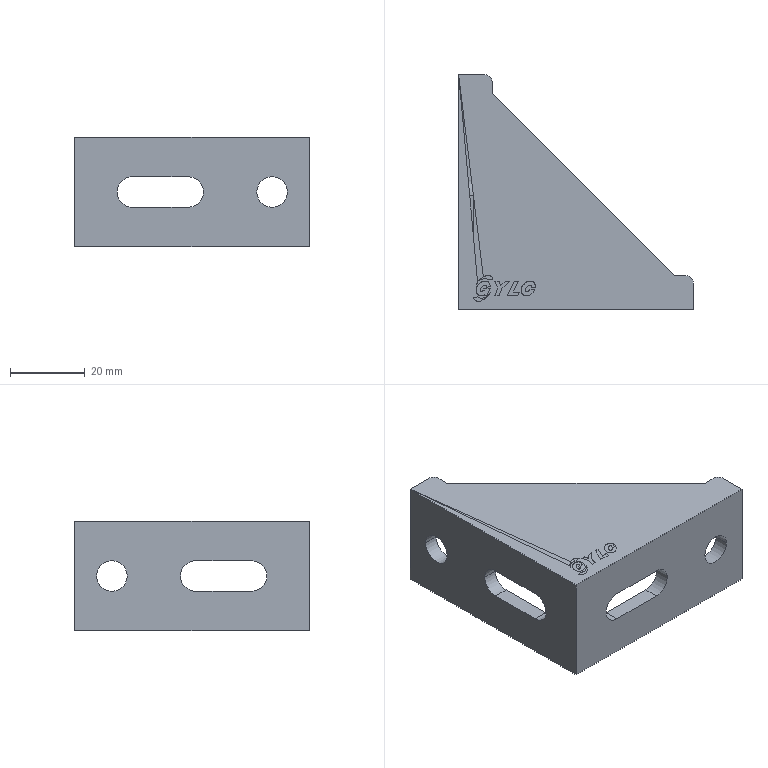Part | NX | features BREP 1 | 1 solid | 78 faces | box 63 x 63 x 29.5 mm | volume 19619 mm3 | plane 48 | spline 17 | cylinder 13 | commonest cylinder face diameters 8.2 x10 4 x2 3.523 x1